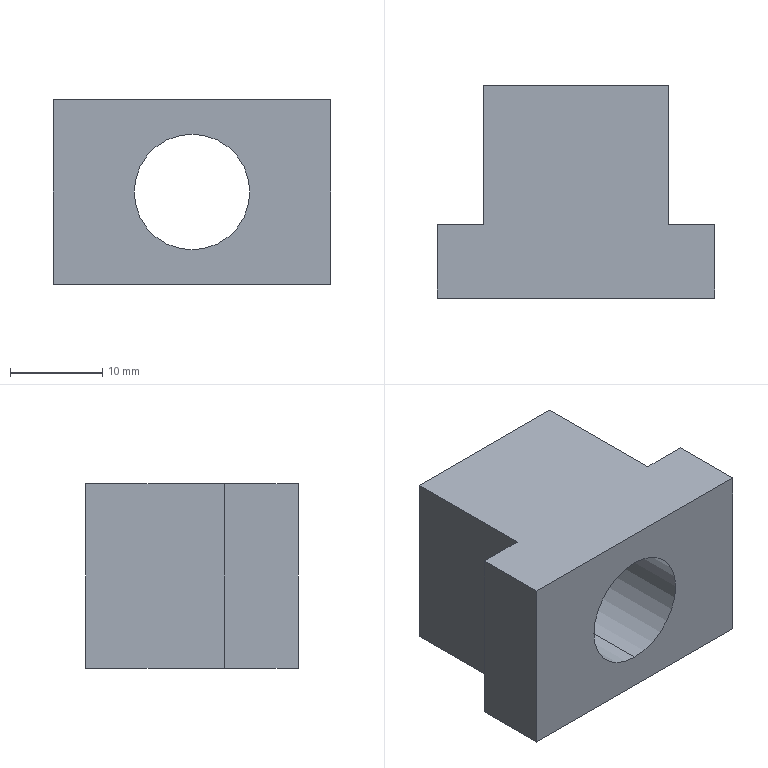Part | STEP file | A14-027 | 1 solid | 12 faces | box 30 x 23 x 20 mm | volume 7977 mm3 | plane 10 | cylinder 2 | commonest cylinder face diameters 12.5 x2
STEP:
#1=CARTESIAN_POINT('',(0.,0.,0.));
#2=DIRECTION('',(0.,0.,1.));
#3=DIRECTION('',(1.,0.,0.));
#4=AXIS2_PLACEMENT_3D('',#1,#2,#3);
#5=CARTESIAN_POINT('',(0.,0.,6.25));
#6=VERTEX_POINT('',#5);
#7=CARTESIAN_POINT('',(0.,23.,6.25));
#8=VERTEX_POINT('',#7);
#9=CARTESIAN_POINT('',(0.,23.,6.25));
#10=DIRECTION('',(0.,1.,0.));
#11=VECTOR('',#10,1.);
#12=LINE('',#9,#11);
#13=CARTESIAN_POINT('',(0.,23.,0.));
#14=DIRECTION('',(0.,1.,0.));
#15=DIRECTION('',(0.,0.,1.));
#16=AXIS2_PLACEMENT_3D('',#13,#14,#15);
#17=CYLINDRICAL_SURFACE('',#16,6.25);
#18=CARTESIAN_POINT('',(6.283,0.));
#19=DIRECTION('',(0.,1.));
#20=VECTOR('',#19,1.);
#21=LINE('',#18,#20);
#22=(GEOMETRIC_REPRESENTATION_CONTEXT(2)PARAMETRIC_REPRESENTATION_CONTEXT()REPRESENTATION_CONTEXT('',''));
#23=DEFINITIONAL_REPRESENTATION('',(#21),#22);
#24=PCURVE('',#17,#23);
#25=CARTESIAN_POINT('',(0.,23.,0.));
#26=DIRECTION('',(0.,1.,0.));
#27=DIRECTION('',(0.,0.,1.));
#28=AXIS2_PLACEMENT_3D('',#25,#26,#27);
#29=CYLINDRICAL_SURFACE('',#28,6.25);
#30=CARTESIAN_POINT('',(0.,0.));
#31=DIRECTION('',(0.,1.));
#32=VECTOR('',#31,1.);
#33=LINE('',#30,#32);
#34=(GEOMETRIC_REPRESENTATION_CONTEXT(2)PARAMETRIC_REPRESENTATION_CONTEXT()REPRESENTATION_CONTEXT('',''));
#35=DEFINITIONAL_REPRESENTATION('',(#33),#34);
#36=PCURVE('',#29,#35);
#37=SURFACE_CURVE('',#12,(#24,#36),.PCURVE_S1.);
#38=EDGE_CURVE('',#6,#8,#37,.T.);
#39=ORIENTED_EDGE('',*,*,#38,.T.);
#40=CARTESIAN_POINT('',(0.,23.,-6.25));
#41=VERTEX_POINT('',#40);
#42=CARTESIAN_POINT('',(0.,23.,0.));
#43=DIRECTION('',(0.,1.,0.));
#44=DIRECTION('',(0.,0.,1.));
#45=AXIS2_PLACEMENT_3D('',#42,#43,#44);
#46=CIRCLE('',#45,6.25);
#47=CARTESIAN_POINT('',(0.,0.));
#48=DIRECTION('',(1.,0.));
#49=VECTOR('',#48,1.);
#50=LINE('',#47,#49);
#51=(GEOMETRIC_REPRESENTATION_CONTEXT(2)PARAMETRIC_REPRESENTATION_CONTEXT()REPRESENTATION_CONTEXT('',''));
#52=DEFINITIONAL_REPRESENTATION('',(#50),#51);
#53=PCURVE('',#17,#52);
#54=CARTESIAN_POINT('',(10.,23.,10.));
#55=DIRECTION('',(0.,-1.,0.));
#56=DIRECTION('',(0.,0.,-1.));
#57=AXIS2_PLACEMENT_3D('',#54,#55,#56);
#58=PLANE('',#57);
#59=CARTESIAN_POINT('',(3.75,-10.));
#60=CARTESIAN_POINT('',(3.75,0.8253));
#61=CARTESIAN_POINT('',(13.125,-4.587));
#62=CARTESIAN_POINT('',(22.5,-10.));
#63=CARTESIAN_POINT('',(13.125,-15.413));
#64=CARTESIAN_POINT('',(3.75,-20.825));
#65=CARTESIAN_POINT('',(3.75,-10.));
#66=(BOUNDED_CURVE()B_SPLINE_CURVE(2,(#59,#60,#61,#62,#63,#64,#65),.UNSPECIFIED.,.T.,.F.)B_SPLINE_CURVE_WITH_KNOTS((1,2,2,2,2,1),(-2.094,0.,2.094,4.189,6.283,8.378),.UNSPECIFIED.)CURVE()GEOMETRIC_REPRESENTATION_ITEM()RATIONAL_B_SPLINE_CURVE((1.,0.5,1.,0.5,1.,0.5,1.))REPRESENTATION_ITEM(''));
#67=(GEOMETRIC_REPRESENTATION_CONTEXT(2)PARAMETRIC_REPRESENTATION_CONTEXT()REPRESENTATION_CONTEXT('',''));
#68=DEFINITIONAL_REPRESENTATION('',(#66),#67);
#69=PCURVE('',#58,#68);
#70=SURFACE_CURVE('',#46,(#53,#69),.PCURVE_S1.);
#71=EDGE_CURVE('',#41,#8,#70,.T.);
#72=ORIENTED_EDGE('',*,*,#71,.F.);
#73=CARTESIAN_POINT('',(0.,0.,-6.25));
#74=VERTEX_POINT('',#73);
#75=CARTESIAN_POINT('',(0.,23.,-6.25));
#76=DIRECTION('',(0.,1.,0.));
#77=VECTOR('',#76,1.);
#78=LINE('',#75,#77);
#79=CARTESIAN_POINT('',(3.142,0.));
#80=DIRECTION('',(0.,1.));
#81=VECTOR('',#80,1.);
#82=LINE('',#79,#81);
#83=(GEOMETRIC_REPRESENTATION_CONTEXT(2)PARAMETRIC_REPRESENTATION_CONTEXT()REPRESENTATION_CONTEXT('',''));
#84=DEFINITIONAL_REPRESENTATION('',(#82),#83);
#85=PCURVE('',#17,#84);
#86=CARTESIAN_POINT('',(3.142,0.));
#87=DIRECTION('',(0.,1.));
#88=VECTOR('',#87,1.);
#89=LINE('',#86,#88);
#90=(GEOMETRIC_REPRESENTATION_CONTEXT(2)PARAMETRIC_REPRESENTATION_CONTEXT()REPRESENTATION_CONTEXT('',''));
#91=DEFINITIONAL_REPRESENTATION('',(#89),#90);
#92=PCURVE('',#29,#91);
#93=SURFACE_CURVE('',#78,(#85,#92),.PCURVE_S1.);
#94=EDGE_CURVE('',#74,#41,#93,.T.);
#95=ORIENTED_EDGE('',*,*,#94,.F.);
#96=CARTESIAN_POINT('',(0.,0.,0.));
#97=DIRECTION('',(0.,1.,0.));
#98=DIRECTION('',(0.,0.,1.));
#99=AXIS2_PLACEMENT_3D('',#96,#97,#98);
#100=CIRCLE('',#99,6.25);
#101=CARTESIAN_POINT('',(0.,-23.));
#102=DIRECTION('',(1.,0.));
#103=VECTOR('',#102,1.);
#104=LINE('',#101,#103);
#105=(GEOMETRIC_REPRESENTATION_CONTEXT(2)PARAMETRIC_REPRESENTATION_CONTEXT()REPRESENTATION_CONTEXT('',''));
#106=DEFINITIONAL_REPRESENTATION('',(#104),#105);
#107=PCURVE('',#17,#106);
#108=CARTESIAN_POINT('',(-15.,0.,10.));
#109=DIRECTION('',(0.,1.,0.));
#110=DIRECTION('',(0.,0.,1.));
#111=AXIS2_PLACEMENT_3D('',#108,#109,#110);
#112=PLANE('',#111);
#113=CARTESIAN_POINT('',(-10.,15.));
#114=DIRECTION('',(1.,0.));
#115=AXIS2_PLACEMENT_2D('',#113,#114);
#116=CIRCLE('',#115,6.25);
#117=(GEOMETRIC_REPRESENTATION_CONTEXT(2)PARAMETRIC_REPRESENTATION_CONTEXT()REPRESENTATION_CONTEXT('',''));
#118=DEFINITIONAL_REPRESENTATION('',(#116),#117);
#119=PCURVE('',#112,#118);
#120=SURFACE_CURVE('',#100,(#107,#119),.PCURVE_S1.);
#121=EDGE_CURVE('',#74,#6,#120,.T.);
#122=ORIENTED_EDGE('',*,*,#121,.T.);
#123=EDGE_LOOP('',(#39,#72,#95,#122));
#124=FACE_BOUND('',#123,.F.);
#125=ADVANCED_FACE('',(#124),#17,.F.);
#126=CARTESIAN_POINT('',(15.,0.,-10.));
#127=VERTEX_POINT('',#126);
#128=CARTESIAN_POINT('',(15.,8.,-10.));
#129=VERTEX_POINT('',#128);
#130=CARTESIAN_POINT('',(15.,0.,-10.));
#131=DIRECTION('',(0.,1.,0.));
#132=VECTOR('',#131,1.);
#133=LINE('',#130,#132);
#134=CARTESIAN_POINT('',(15.,0.,10.));
#135=DIRECTION('',(-1.,0.,0.));
#136=DIRECTION('',(0.,0.,1.));
#137=AXIS2_PLACEMENT_3D('',#134,#135,#136);
#138=PLANE('',#137);
#139=CARTESIAN_POINT('',(-20.,0.));
#140=DIRECTION('',(0.,1.));
#141=VECTOR('',#140,1.);
#142=LINE('',#139,#141);
#143=(GEOMETRIC_REPRESENTATION_CONTEXT(2)PARAMETRIC_REPRESENTATION_CONTEXT()REPRESENTATION_CONTEXT('',''));
#144=DEFINITIONAL_REPRESENTATION('',(#142),#143);
#145=PCURVE('',#138,#144);
#146=CARTESIAN_POINT('',(0.,0.,-10.));
#147=DIRECTION('',(0.,0.,1.));
#148=DIRECTION('',(1.,0.,0.));
#149=AXIS2_PLACEMENT_3D('',#146,#147,#148);
#150=PLANE('',#149);
#151=CARTESIAN_POINT('',(15.,0.));
#152=DIRECTION('',(0.,1.));
#153=VECTOR('',#152,1.);
#154=LINE('',#151,#153);
#155=(GEOMETRIC_REPRESENTATION_CONTEXT(2)PARAMETRIC_REPRESENTATION_CONTEXT()REPRESENTATION_CONTEXT('',''));
#156=DEFINITIONAL_REPRESENTATION('',(#154),#155);
#157=PCURVE('',#150,#156);
#158=SURFACE_CURVE('',#133,(#145,#157),.PCURVE_S1.);
#159=EDGE_CURVE('',#127,#129,#158,.T.);
#160=ORIENTED_EDGE('',*,*,#159,.T.);
#161=CARTESIAN_POINT('',(15.,8.,10.));
#162=VERTEX_POINT('',#161);
#163=CARTESIAN_POINT('',(15.,8.,10.));
#164=DIRECTION('',(0.,0.,-1.));
#165=VECTOR('',#164,1.);
#166=LINE('',#163,#165);
#167=CARTESIAN_POINT('',(0.,8.));
#168=DIRECTION('',(-1.,0.));
#169=VECTOR('',#168,1.);
#170=LINE('',#167,#169);
#171=(GEOMETRIC_REPRESENTATION_CONTEXT(2)PARAMETRIC_REPRESENTATION_CONTEXT()REPRESENTATION_CONTEXT('',''));
#172=DEFINITIONAL_REPRESENTATION('',(#170),#171);
#173=PCURVE('',#138,#172);
#174=CARTESIAN_POINT('',(15.,8.,10.));
#175=DIRECTION('',(0.,-1.,0.));
#176=DIRECTION('',(1.,0.,0.));
#177=AXIS2_PLACEMENT_3D('',#174,#175,#176);
#178=PLANE('',#177);
#179=CARTESIAN_POINT('',(0.,0.));
#180=DIRECTION('',(0.,-1.));
#181=VECTOR('',#180,1.);
#182=LINE('',#179,#181);
#183=(GEOMETRIC_REPRESENTATION_CONTEXT(2)PARAMETRIC_REPRESENTATION_CONTEXT()REPRESENTATION_CONTEXT('',''));
#184=DEFINITIONAL_REPRESENTATION('',(#182),#183);
#185=PCURVE('',#178,#184);
#186=SURFACE_CURVE('',#166,(#173,#185),.PCURVE_S1.);
#187=EDGE_CURVE('',#162,#129,#186,.T.);
#188=ORIENTED_EDGE('',*,*,#187,.F.);
#189=CARTESIAN_POINT('',(15.,0.,10.));
#190=VERTEX_POINT('',#189);
#191=CARTESIAN_POINT('',(15.,0.,10.));
#192=DIRECTION('',(0.,1.,0.));
#193=VECTOR('',#192,1.);
#194=LINE('',#191,#193);
#195=CARTESIAN_POINT('',(0.,0.));
#196=DIRECTION('',(0.,1.));
#197=VECTOR('',#196,1.);
#198=LINE('',#195,#197);
#199=(GEOMETRIC_REPRESENTATION_CONTEXT(2)PARAMETRIC_REPRESENTATION_CONTEXT()REPRESENTATION_CONTEXT('',''));
#200=DEFINITIONAL_REPRESENTATION('',(#198),#199);
#201=PCURVE('',#138,#200);
#202=CARTESIAN_POINT('',(0.,0.,10.));
#203=DIRECTION('',(0.,0.,1.));
#204=DIRECTION('',(1.,0.,0.));
#205=AXIS2_PLACEMENT_3D('',#202,#203,#204);
#206=PLANE('',#205);
#207=CARTESIAN_POINT('',(15.,0.));
#208=DIRECTION('',(0.,1.));
#209=VECTOR('',#208,1.);
#210=LINE('',#207,#209);
#211=(GEOMETRIC_REPRESENTATION_CONTEXT(2)PARAMETRIC_REPRESENTATION_CONTEXT()REPRESENTATION_CONTEXT('',''));
#212=DEFINITIONAL_REPRESENTATION('',(#210),#211);
#213=PCURVE('',#206,#212);
#214=SURFACE_CURVE('',#194,(#201,#213),.PCURVE_S1.);
#215=EDGE_CURVE('',#190,#162,#214,.T.);
#216=ORIENTED_EDGE('',*,*,#215,.F.);
#217=CARTESIAN_POINT('',(15.,0.,10.));
#218=DIRECTION('',(0.,0.,-1.));
#219=VECTOR('',#218,1.);
#220=LINE('',#217,#219);
#221=CARTESIAN_POINT('',(0.,0.));
#222=DIRECTION('',(-1.,0.));
#223=VECTOR('',#222,1.);
#224=LINE('',#221,#223);
#225=(GEOMETRIC_REPRESENTATION_CONTEXT(2)PARAMETRIC_REPRESENTATION_CONTEXT()REPRESENTATION_CONTEXT('',''));
#226=DEFINITIONAL_REPRESENTATION('',(#224),#225);
#227=PCURVE('',#138,#226);
#228=CARTESIAN_POINT('',(0.,30.));
#229=DIRECTION('',(-1.,0.));
#230=VECTOR('',#229,1.);
#231=LINE('',#228,#230);
#232=(GEOMETRIC_REPRESENTATION_CONTEXT(2)PARAMETRIC_REPRESENTATION_CONTEXT()REPRESENTATION_CONTEXT('',''));
#233=DEFINITIONAL_REPRESENTATION('',(#231),#232);
#234=PCURVE('',#112,#233);
#235=SURFACE_CURVE('',#220,(#227,#234),.PCURVE_S1.);
#236=EDGE_CURVE('',#190,#127,#235,.T.);
#237=ORIENTED_EDGE('',*,*,#236,.T.);
#238=EDGE_LOOP('',(#160,#188,#216,#237));
#239=FACE_BOUND('',#238,.T.);
#240=ADVANCED_FACE('',(#239),#138,.F.);
#241=CARTESIAN_POINT('',(10.,8.,-10.));
#242=VERTEX_POINT('',#241);
#243=CARTESIAN_POINT('',(15.,8.,-10.));
#244=DIRECTION('',(-1.,0.,0.));
#245=VECTOR('',#244,1.);
#246=LINE('',#243,#245);
#247=CARTESIAN_POINT('',(0.,-20.));
#248=DIRECTION('',(-1.,0.));
#249=VECTOR('',#248,1.);
#250=LINE('',#247,#249);
#251=(GEOMETRIC_REPRESENTATION_CONTEXT(2)PARAMETRIC_REPRESENTATION_CONTEXT()REPRESENTATION_CONTEXT('',''));
#252=DEFINITIONAL_REPRESENTATION('',(#250),#251);
#253=PCURVE('',#178,#252);
#254=CARTESIAN_POINT('',(15.,8.));
#255=DIRECTION('',(-1.,0.));
#256=VECTOR('',#255,1.);
#257=LINE('',#254,#256);
#258=(GEOMETRIC_REPRESENTATION_CONTEXT(2)PARAMETRIC_REPRESENTATION_CONTEXT()REPRESENTATION_CONTEXT('',''));
#259=DEFINITIONAL_REPRESENTATION('',(#257),#258);
#260=PCURVE('',#150,#259);
#261=SURFACE_CURVE('',#246,(#253,#260),.PCURVE_S1.);
#262=EDGE_CURVE('',#129,#242,#261,.T.);
#263=ORIENTED_EDGE('',*,*,#262,.T.);
#264=CARTESIAN_POINT('',(10.,8.,10.));
#265=VERTEX_POINT('',#264);
#266=CARTESIAN_POINT('',(10.,8.,10.));
#267=DIRECTION('',(0.,0.,-1.));
#268=VECTOR('',#267,1.);
#269=LINE('',#266,#268);
#270=CARTESIAN_POINT('',(-5.,0.));
#271=DIRECTION('',(0.,-1.));
#272=VECTOR('',#271,1.);
#273=LINE('',#270,#272);
#274=(GEOMETRIC_REPRESENTATION_CONTEXT(2)PARAMETRIC_REPRESENTATION_CONTEXT()REPRESENTATION_CONTEXT('',''));
#275=DEFINITIONAL_REPRESENTATION('',(#273),#274);
#276=PCURVE('',#178,#275);
#277=CARTESIAN_POINT('',(10.,8.,10.));
#278=DIRECTION('',(-1.,0.,0.));
#279=DIRECTION('',(0.,0.,1.));
#280=AXIS2_PLACEMENT_3D('',#277,#278,#279);
#281=PLANE('',#280);
#282=CARTESIAN_POINT('',(0.,0.));
#283=DIRECTION('',(-1.,0.));
#284=VECTOR('',#283,1.);
#285=LINE('',#282,#284);
#286=(GEOMETRIC_REPRESENTATION_CONTEXT(2)PARAMETRIC_REPRESENTATION_CONTEXT()REPRESENTATION_CONTEXT('',''));
#287=DEFINITIONAL_REPRESENTATION('',(#285),#286);
#288=PCURVE('',#281,#287);
#289=SURFACE_CURVE('',#269,(#276,#288),.PCURVE_S1.);
#290=EDGE_CURVE('',#265,#242,#289,.T.);
#291=ORIENTED_EDGE('',*,*,#290,.F.);
#292=CARTESIAN_POINT('',(15.,8.,10.));
#293=DIRECTION('',(-1.,0.,0.));
#294=VECTOR('',#293,1.);
#295=LINE('',#292,#294);
#296=CARTESIAN_POINT('',(0.,0.));
#297=DIRECTION('',(-1.,0.));
#298=VECTOR('',#297,1.);
#299=LINE('',#296,#298);
#300=(GEOMETRIC_REPRESENTATION_CONTEXT(2)PARAMETRIC_REPRESENTATION_CONTEXT()REPRESENTATION_CONTEXT('',''));
#301=DEFINITIONAL_REPRESENTATION('',(#299),#300);
#302=PCURVE('',#178,#301);
#303=CARTESIAN_POINT('',(15.,8.));
#304=DIRECTION('',(-1.,0.));
#305=VECTOR('',#304,1.);
#306=LINE('',#303,#305);
#307=(GEOMETRIC_REPRESENTATION_CONTEXT(2)PARAMETRIC_REPRESENTATION_CONTEXT()REPRESENTATION_CONTEXT('',''));
#308=DEFINITIONAL_REPRESENTATION('',(#306),#307);
#309=PCURVE('',#206,#308);
#310=SURFACE_CURVE('',#295,(#302,#309),.PCURVE_S1.);
#311=EDGE_CURVE('',#162,#265,#310,.T.);
#312=ORIENTED_EDGE('',*,*,#311,.F.);
#313=ORIENTED_EDGE('',*,*,#187,.T.);
#314=EDGE_LOOP('',(#263,#291,#312,#313));
#315=FACE_BOUND('',#314,.T.);
#316=ADVANCED_FACE('',(#315),#178,.F.);
#317=CARTESIAN_POINT('',(10.,23.,-10.));
#318=VERTEX_POINT('',#317);
#319=CARTESIAN_POINT('',(10.,8.,-10.));
#320=DIRECTION('',(0.,1.,0.));
#321=VECTOR('',#320,1.);
#322=LINE('',#319,#321);
#323=CARTESIAN_POINT('',(-20.,0.));
#324=DIRECTION('',(0.,1.));
#325=VECTOR('',#324,1.);
#326=LINE('',#323,#325);
#327=(GEOMETRIC_REPRESENTATION_CONTEXT(2)PARAMETRIC_REPRESENTATION_CONTEXT()REPRESENTATION_CONTEXT('',''));
#328=DEFINITIONAL_REPRESENTATION('',(#326),#327);
#329=PCURVE('',#281,#328);
#330=CARTESIAN_POINT('',(10.,8.));
#331=DIRECTION('',(0.,1.));
#332=VECTOR('',#331,1.);
#333=LINE('',#330,#332);
#334=(GEOMETRIC_REPRESENTATION_CONTEXT(2)PARAMETRIC_REPRESENTATION_CONTEXT()REPRESENTATION_CONTEXT('',''));
#335=DEFINITIONAL_REPRESENTATION('',(#333),#334);
#336=PCURVE('',#150,#335);
#337=SURFACE_CURVE('',#322,(#329,#336),.PCURVE_S1.);
#338=EDGE_CURVE('',#242,#318,#337,.T.);
#339=ORIENTED_EDGE('',*,*,#338,.T.);
#340=CARTESIAN_POINT('',(10.,23.,10.));
#341=VERTEX_POINT('',#340);
#342=CARTESIAN_POINT('',(10.,23.,10.));
#343=DIRECTION('',(0.,0.,-1.));
#344=VECTOR('',#343,1.);
#345=LINE('',#342,#344);
#346=CARTESIAN_POINT('',(0.,15.));
#347=DIRECTION('',(-1.,0.));
#348=VECTOR('',#347,1.);
#349=LINE('',#346,#348);
#350=(GEOMETRIC_REPRESENTATION_CONTEXT(2)PARAMETRIC_REPRESENTATION_CONTEXT()REPRESENTATION_CONTEXT('',''));
#351=DEFINITIONAL_REPRESENTATION('',(#349),#350);
#352=PCURVE('',#281,#351);
#353=CARTESIAN_POINT('',(0.,0.));
#354=DIRECTION('',(1.,0.));
#355=VECTOR('',#354,1.);
#356=LINE('',#353,#355);
#357=(GEOMETRIC_REPRESENTATION_CONTEXT(2)PARAMETRIC_REPRESENTATION_CONTEXT()REPRESENTATION_CONTEXT('',''));
#358=DEFINITIONAL_REPRESENTATION('',(#356),#357);
#359=PCURVE('',#58,#358);
#360=SURFACE_CURVE('',#345,(#352,#359),.PCURVE_S1.);
#361=EDGE_CURVE('',#341,#318,#360,.T.);
#362=ORIENTED_EDGE('',*,*,#361,.F.);
#363=CARTESIAN_POINT('',(10.,8.,10.));
#364=DIRECTION('',(0.,1.,0.));
#365=VECTOR('',#364,1.);
#366=LINE('',#363,#365);
#367=CARTESIAN_POINT('',(0.,0.));
#368=DIRECTION('',(0.,1.));
#369=VECTOR('',#368,1.);
#370=LINE('',#367,#369);
#371=(GEOMETRIC_REPRESENTATION_CONTEXT(2)PARAMETRIC_REPRESENTATION_CONTEXT()REPRESENTATION_CONTEXT('',''));
#372=DEFINITIONAL_REPRESENTATION('',(#370),#371);
#373=PCURVE('',#281,#372);
#374=CARTESIAN_POINT('',(10.,8.));
#375=DIRECTION('',(0.,1.));
#376=VECTOR('',#375,1.);
#377=LINE('',#374,#376);
#378=(GEOMETRIC_REPRESENTATION_CONTEXT(2)PARAMETRIC_REPRESENTATION_CONTEXT()REPRESENTATION_CONTEXT('',''));
#379=DEFINITIONAL_REPRESENTATION('',(#377),#378);
#380=PCURVE('',#206,#379);
#381=SURFACE_CURVE('',#366,(#373,#380),.PCURVE_S1.);
#382=EDGE_CURVE('',#265,#341,#381,.T.);
#383=ORIENTED_EDGE('',*,*,#382,.F.);
#384=ORIENTED_EDGE('',*,*,#290,.T.);
#385=EDGE_LOOP('',(#339,#362,#383,#384));
#386=FACE_BOUND('',#385,.T.);
#387=ADVANCED_FACE('',(#386),#281,.F.);
#388=CARTESIAN_POINT('',(0.,23.,0.));
#389=DIRECTION('',(0.,1.,0.));
#390=DIRECTION('',(0.,0.,1.));
#391=AXIS2_PLACEMENT_3D('',#388,#389,#390);
#392=CIRCLE('',#391,6.25);
#393=CARTESIAN_POINT('',(3.75,-10.));
#394=CARTESIAN_POINT('',(3.75,0.8253));
#395=CARTESIAN_POINT('',(13.125,-4.587));
#396=CARTESIAN_POINT('',(22.5,-10.));
#397=CARTESIAN_POINT('',(13.125,-15.413));
#398=CARTESIAN_POINT('',(3.75,-20.825));
#399=CARTESIAN_POINT('',(3.75,-10.));
#400=(BOUNDED_CURVE()B_SPLINE_CURVE(2,(#393,#394,#395,#396,#397,#398,#399),.UNSPECIFIED.,.T.,.F.)B_SPLINE_CURVE_WITH_KNOTS((1,2,2,2,2,1),(-2.094,0.,2.094,4.189,6.283,8.378),.UNSPECIFIED.)CURVE()GEOMETRIC_REPRESENTATION_ITEM()RATIONAL_B_SPLINE_CURVE((1.,0.5,1.,0.5,1.,0.5,1.))REPRESENTATION_ITEM(''));
#401=(GEOMETRIC_REPRESENTATION_CONTEXT(2)PARAMETRIC_REPRESENTATION_CONTEXT()REPRESENTATION_CONTEXT('',''));
#402=DEFINITIONAL_REPRESENTATION('',(#400),#401);
#403=PCURVE('',#58,#402);
#404=CARTESIAN_POINT('',(0.,0.));
#405=DIRECTION('',(1.,0.));
#406=VECTOR('',#405,1.);
#407=LINE('',#404,#406);
#408=(GEOMETRIC_REPRESENTATION_CONTEXT(2)PARAMETRIC_REPRESENTATION_CONTEXT()REPRESENTATION_CONTEXT('',''));
#409=DEFINITIONAL_REPRESENTATION('',(#407),#408);
#410=PCURVE('',#29,#409);
#411=SURFACE_CURVE('',#392,(#403,#410),.PCURVE_S1.);
#412=EDGE_CURVE('',#8,#41,#411,.T.);
#413=ORIENTED_EDGE('',*,*,#412,.F.);
#414=ORIENTED_EDGE('',*,*,#71,.F.);
#415=EDGE_LOOP('',(#413,#414));
#416=FACE_BOUND('',#415,.T.);
#417=CARTESIAN_POINT('',(-10.,23.,-10.));
#418=VERTEX_POINT('',#417);
#419=CARTESIAN_POINT('',(10.,23.,-10.));
#420=DIRECTION('',(-1.,0.,0.));
#421=VECTOR('',#420,1.);
#422=LINE('',#419,#421);
#423=CARTESIAN_POINT('',(20.,0.));
#424=DIRECTION('',(0.,-1.));
#425=VECTOR('',#424,1.);
#426=LINE('',#423,#425);
#427=(GEOMETRIC_REPRESENTATION_CONTEXT(2)PARAMETRIC_REPRESENTATION_CONTEXT()REPRESENTATION_CONTEXT('',''));
#428=DEFINITIONAL_REPRESENTATION('',(#426),#427);
#429=PCURVE('',#58,#428);
#430=CARTESIAN_POINT('',(10.,23.));
#431=DIRECTION('',(-1.,0.));
#432=VECTOR('',#431,1.);
#433=LINE('',#430,#432);
#434=(GEOMETRIC_REPRESENTATION_CONTEXT(2)PARAMETRIC_REPRESENTATION_CONTEXT()REPRESENTATION_CONTEXT('',''));
#435=DEFINITIONAL_REPRESENTATION('',(#433),#434);
#436=PCURVE('',#150,#435);
#437=SURFACE_CURVE('',#422,(#429,#436),.PCURVE_S1.);
#438=EDGE_CURVE('',#318,#418,#437,.T.);
#439=ORIENTED_EDGE('',*,*,#438,.T.);
#440=CARTESIAN_POINT('',(-10.,23.,10.));
#441=VERTEX_POINT('',#440);
#442=CARTESIAN_POINT('',(-10.,23.,10.));
#443=DIRECTION('',(0.,0.,-1.));
#444=VECTOR('',#443,1.);
#445=LINE('',#442,#444);
#446=CARTESIAN_POINT('',(0.,-20.));
#447=DIRECTION('',(1.,0.));
#448=VECTOR('',#447,1.);
#449=LINE('',#446,#448);
#450=(GEOMETRIC_REPRESENTATION_CONTEXT(2)PARAMETRIC_REPRESENTATION_CONTEXT()REPRESENTATION_CONTEXT('',''));
#451=DEFINITIONAL_REPRESENTATION('',(#449),#450);
#452=PCURVE('',#58,#451);
#453=CARTESIAN_POINT('',(-10.,23.,10.));
#454=DIRECTION('',(1.,0.,0.));
#455=DIRECTION('',(0.,1.,0.));
#456=AXIS2_PLACEMENT_3D('',#453,#454,#455);
#457=PLANE('',#456);
#458=CARTESIAN_POINT('',(0.,0.));
#459=DIRECTION('',(0.,-1.));
#460=VECTOR('',#459,1.);
#461=LINE('',#458,#460);
#462=(GEOMETRIC_REPRESENTATION_CONTEXT(2)PARAMETRIC_REPRESENTATION_CONTEXT()REPRESENTATION_CONTEXT('',''));
#463=DEFINITIONAL_REPRESENTATION('',(#461),#462);
#464=PCURVE('',#457,#463);
#465=SURFACE_CURVE('',#445,(#452,#464),.PCURVE_S1.);
#466=EDGE_CURVE('',#441,#418,#465,.T.);
#467=ORIENTED_EDGE('',*,*,#466,.F.);
#468=CARTESIAN_POINT('',(10.,23.,10.));
#469=DIRECTION('',(-1.,0.,0.));
#470=VECTOR('',#469,1.);
#471=LINE('',#468,#470);
#472=CARTESIAN_POINT('',(0.,0.));
#473=DIRECTION('',(0.,-1.));
#474=VECTOR('',#473,1.);
#475=LINE('',#472,#474);
#476=(GEOMETRIC_REPRESENTATION_CONTEXT(2)PARAMETRIC_REPRESENTATION_CONTEXT()REPRESENTATION_CONTEXT('',''));
#477=DEFINITIONAL_REPRESENTATION('',(#475),#476);
#478=PCURVE('',#58,#477);
#479=CARTESIAN_POINT('',(10.,23.));
#480=DIRECTION('',(-1.,0.));
#481=VECTOR('',#480,1.);
#482=LINE('',#479,#481);
#483=(GEOMETRIC_REPRESENTATION_CONTEXT(2)PARAMETRIC_REPRESENTATION_CONTEXT()REPRESENTATION_CONTEXT('',''));
#484=DEFINITIONAL_REPRESENTATION('',(#482),#483);
#485=PCURVE('',#206,#484);
#486=SURFACE_CURVE('',#471,(#478,#485),.PCURVE_S1.);
#487=EDGE_CURVE('',#341,#441,#486,.T.);
#488=ORIENTED_EDGE('',*,*,#487,.F.);
#489=ORIENTED_EDGE('',*,*,#361,.T.);
#490=EDGE_LOOP('',(#439,#467,#488,#489));
#491=FACE_BOUND('',#490,.T.);
#492=ADVANCED_FACE('',(#416,#491),#58,.F.);
#493=CARTESIAN_POINT('',(-10.,8.,-10.));
#494=VERTEX_POINT('',#493);
#495=CARTESIAN_POINT('',(-10.,23.,-10.));
#496=DIRECTION('',(0.,-1.,0.));
#497=VECTOR('',#496,1.);
#498=LINE('',#495,#497);
#499=CARTESIAN_POINT('',(0.,-20.));
#500=DIRECTION('',(-1.,0.));
#501=VECTOR('',#500,1.);
#502=LINE('',#499,#501);
#503=(GEOMETRIC_REPRESENTATION_CONTEXT(2)PARAMETRIC_REPRESENTATION_CONTEXT()REPRESENTATION_CONTEXT('',''));
#504=DEFINITIONAL_REPRESENTATION('',(#502),#503);
#505=PCURVE('',#457,#504);
#506=CARTESIAN_POINT('',(-10.,23.));
#507=DIRECTION('',(0.,-1.));
#508=VECTOR('',#507,1.);
#509=LINE('',#506,#508);
#510=(GEOMETRIC_REPRESENTATION_CONTEXT(2)PARAMETRIC_REPRESENTATION_CONTEXT()REPRESENTATION_CONTEXT('',''));
#511=DEFINITIONAL_REPRESENTATION('',(#509),#510);
#512=PCURVE('',#150,#511);
#513=SURFACE_CURVE('',#498,(#505,#512),.PCURVE_S1.);
#514=EDGE_CURVE('',#418,#494,#513,.T.);
#515=ORIENTED_EDGE('',*,*,#514,.T.);
#516=CARTESIAN_POINT('',(-10.,8.,10.));
#517=VERTEX_POINT('',#516);
#518=CARTESIAN_POINT('',(-10.,8.,10.));
#519=DIRECTION('',(0.,0.,-1.));
#520=VECTOR('',#519,1.);
#521=LINE('',#518,#520);
#522=CARTESIAN_POINT('',(-15.,0.));
#523=DIRECTION('',(0.,-1.));
#524=VECTOR('',#523,1.);
#525=LINE('',#522,#524);
#526=(GEOMETRIC_REPRESENTATION_CONTEXT(2)PARAMETRIC_REPRESENTATION_CONTEXT()REPRESENTATION_CONTEXT('',''));
#527=DEFINITIONAL_REPRESENTATION('',(#525),#526);
#528=PCURVE('',#457,#527);
#529=CARTESIAN_POINT('',(-10.,8.,10.));
#530=DIRECTION('',(0.,-1.,0.));
#531=DIRECTION('',(1.,0.,0.));
#532=AXIS2_PLACEMENT_3D('',#529,#530,#531);
#533=PLANE('',#532);
#534=CARTESIAN_POINT('',(0.,0.));
#535=DIRECTION('',(0.,-1.));
#536=VECTOR('',#535,1.);
#537=LINE('',#534,#536);
#538=(GEOMETRIC_REPRESENTATION_CONTEXT(2)PARAMETRIC_REPRESENTATION_CONTEXT()REPRESENTATION_CONTEXT('',''));
#539=DEFINITIONAL_REPRESENTATION('',(#537),#538);
#540=PCURVE('',#533,#539);
#541=SURFACE_CURVE('',#521,(#528,#540),.PCURVE_S1.);
#542=EDGE_CURVE('',#517,#494,#541,.T.);
#543=ORIENTED_EDGE('',*,*,#542,.F.);
#544=CARTESIAN_POINT('',(-10.,23.,10.));
#545=DIRECTION('',(0.,-1.,0.));
#546=VECTOR('',#545,1.);
#547=LINE('',#544,#546);
#548=CARTESIAN_POINT('',(0.,0.));
#549=DIRECTION('',(-1.,0.));
#550=VECTOR('',#549,1.);
#551=LINE('',#548,#550);
#552=(GEOMETRIC_REPRESENTATION_CONTEXT(2)PARAMETRIC_REPRESENTATION_CONTEXT()REPRESENTATION_CONTEXT('',''));
#553=DEFINITIONAL_REPRESENTATION('',(#551),#552);
#554=PCURVE('',#457,#553);
#555=CARTESIAN_POINT('',(-10.,23.));
#556=DIRECTION('',(0.,-1.));
#557=VECTOR('',#556,1.);
#558=LINE('',#555,#557);
#559=(GEOMETRIC_REPRESENTATION_CONTEXT(2)PARAMETRIC_REPRESENTATION_CONTEXT()REPRESENTATION_CONTEXT('',''));
#560=DEFINITIONAL_REPRESENTATION('',(#558),#559);
#561=PCURVE('',#206,#560);
#562=SURFACE_CURVE('',#547,(#554,#561),.PCURVE_S1.);
#563=EDGE_CURVE('',#441,#517,#562,.T.);
#564=ORIENTED_EDGE('',*,*,#563,.F.);
#565=ORIENTED_EDGE('',*,*,#466,.T.);
#566=EDGE_LOOP('',(#515,#543,#564,#565));
#567=FACE_BOUND('',#566,.T.);
#568=ADVANCED_FACE('',(#567),#457,.F.);
#569=CARTESIAN_POINT('',(-15.,8.,-10.));
#570=VERTEX_POINT('',#569);
#571=CARTESIAN_POINT('',(-10.,8.,-10.));
#572=DIRECTION('',(-1.,0.,0.));
#573=VECTOR('',#572,1.);
#574=LINE('',#571,#573);
#575=CARTESIAN_POINT('',(0.,-20.));
#576=DIRECTION('',(-1.,0.));
#577=VECTOR('',#576,1.);
#578=LINE('',#575,#577);
#579=(GEOMETRIC_REPRESENTATION_CONTEXT(2)PARAMETRIC_REPRESENTATION_CONTEXT()REPRESENTATION_CONTEXT('',''));
#580=DEFINITIONAL_REPRESENTATION('',(#578),#579);
#581=PCURVE('',#533,#580);
#582=CARTESIAN_POINT('',(-10.,8.));
#583=DIRECTION('',(-1.,0.));
#584=VECTOR('',#583,1.);
#585=LINE('',#582,#584);
#586=(GEOMETRIC_REPRESENTATION_CONTEXT(2)PARAMETRIC_REPRESENTATION_CONTEXT()REPRESENTATION_CONTEXT('',''));
#587=DEFINITIONAL_REPRESENTATION('',(#585),#586);
#588=PCURVE('',#150,#587);
#589=SURFACE_CURVE('',#574,(#581,#588),.PCURVE_S1.);
#590=EDGE_CURVE('',#494,#570,#589,.T.);
#591=ORIENTED_EDGE('',*,*,#590,.T.);
#592=CARTESIAN_POINT('',(-15.,8.,10.));
#593=VERTEX_POINT('',#592);
#594=CARTESIAN_POINT('',(-15.,8.,10.));
#595=DIRECTION('',(0.,0.,-1.));
#596=VECTOR('',#595,1.);
#597=LINE('',#594,#596);
#598=CARTESIAN_POINT('',(-5.,0.));
#599=DIRECTION('',(0.,-1.));
#600=VECTOR('',#599,1.);
#601=LINE('',#598,#600);
#602=(GEOMETRIC_REPRESENTATION_CONTEXT(2)PARAMETRIC_REPRESENTATION_CONTEXT()REPRESENTATION_CONTEXT('',''));
#603=DEFINITIONAL_REPRESENTATION('',(#601),#602);
#604=PCURVE('',#533,#603);
#605=CARTESIAN_POINT('',(-15.,8.,10.));
#606=DIRECTION('',(1.,0.,0.));
#607=DIRECTION('',(0.,1.,0.));
#608=AXIS2_PLACEMENT_3D('',#605,#606,#607);
#609=PLANE('',#608);
#610=CARTESIAN_POINT('',(0.,0.));
#611=DIRECTION('',(0.,-1.));
#612=VECTOR('',#611,1.);
#613=LINE('',#610,#612);
#614=(GEOMETRIC_REPRESENTATION_CONTEXT(2)PARAMETRIC_REPRESENTATION_CONTEXT()REPRESENTATION_CONTEXT('',''));
#615=DEFINITIONAL_REPRESENTATION('',(#613),#614);
#616=PCURVE('',#609,#615);
#617=SURFACE_CURVE('',#597,(#604,#616),.PCURVE_S1.);
#618=EDGE_CURVE('',#593,#570,#617,.T.);
#619=ORIENTED_EDGE('',*,*,#618,.F.);
#620=CARTESIAN_POINT('',(-10.,8.,10.));
#621=DIRECTION('',(-1.,0.,0.));
#622=VECTOR('',#621,1.);
#623=LINE('',#620,#622);
#624=CARTESIAN_POINT('',(0.,0.));
#625=DIRECTION('',(-1.,0.));
#626=VECTOR('',#625,1.);
#627=LINE('',#624,#626);
#628=(GEOMETRIC_REPRESENTATION_CONTEXT(2)PARAMETRIC_REPRESENTATION_CONTEXT()REPRESENTATION_CONTEXT('',''));
#629=DEFINITIONAL_REPRESENTATION('',(#627),#628);
#630=PCURVE('',#533,#629);
#631=CARTESIAN_POINT('',(-10.,8.));
#632=DIRECTION('',(-1.,0.));
#633=VECTOR('',#632,1.);
#634=LINE('',#631,#633);
#635=(GEOMETRIC_REPRESENTATION_CONTEXT(2)PARAMETRIC_REPRESENTATION_CONTEXT()REPRESENTATION_CONTEXT('',''));
#636=DEFINITIONAL_REPRESENTATION('',(#634),#635);
#637=PCURVE('',#206,#636);
#638=SURFACE_CURVE('',#623,(#630,#637),.PCURVE_S1.);
#639=EDGE_CURVE('',#517,#593,#638,.T.);
#640=ORIENTED_EDGE('',*,*,#639,.F.);
#641=ORIENTED_EDGE('',*,*,#542,.T.);
#642=EDGE_LOOP('',(#591,#619,#640,#641));
#643=FACE_BOUND('',#642,.T.);
#644=ADVANCED_FACE('',(#643),#533,.F.);
#645=CARTESIAN_POINT('',(-15.,0.,-10.));
#646=VERTEX_POINT('',#645);
#647=CARTESIAN_POINT('',(-15.,8.,-10.));
#648=DIRECTION('',(0.,-1.,0.));
#649=VECTOR('',#648,1.);
#650=LINE('',#647,#649);
#651=CARTESIAN_POINT('',(0.,-20.));
#652=DIRECTION('',(-1.,0.));
#653=VECTOR('',#652,1.);
#654=LINE('',#651,#653);
#655=(GEOMETRIC_REPRESENTATION_CONTEXT(2)PARAMETRIC_REPRESENTATION_CONTEXT()REPRESENTATION_CONTEXT('',''));
#656=DEFINITIONAL_REPRESENTATION('',(#654),#655);
#657=PCURVE('',#609,#656);
#658=CARTESIAN_POINT('',(-15.,8.));
#659=DIRECTION('',(0.,-1.));
#660=VECTOR('',#659,1.);
#661=LINE('',#658,#660);
#662=(GEOMETRIC_REPRESENTATION_CONTEXT(2)PARAMETRIC_REPRESENTATION_CONTEXT()REPRESENTATION_CONTEXT('',''));
#663=DEFINITIONAL_REPRESENTATION('',(#661),#662);
#664=PCURVE('',#150,#663);
#665=SURFACE_CURVE('',#650,(#657,#664),.PCURVE_S1.);
#666=EDGE_CURVE('',#570,#646,#665,.T.);
#667=ORIENTED_EDGE('',*,*,#666,.T.);
#668=CARTESIAN_POINT('',(-15.,0.,10.));
#669=VERTEX_POINT('',#668);
#670=CARTESIAN_POINT('',(-15.,0.,10.));
#671=DIRECTION('',(0.,0.,-1.));
#672=VECTOR('',#671,1.);
#673=LINE('',#670,#672);
#674=CARTESIAN_POINT('',(-8.,0.));
#675=DIRECTION('',(0.,-1.));
#676=VECTOR('',#675,1.);
#677=LINE('',#674,#676);
#678=(GEOMETRIC_REPRESENTATION_CONTEXT(2)PARAMETRIC_REPRESENTATION_CONTEXT()REPRESENTATION_CONTEXT('',''));
#679=DEFINITIONAL_REPRESENTATION('',(#677),#678);
#680=PCURVE('',#609,#679);
#681=CARTESIAN_POINT('',(0.,0.));
#682=DIRECTION('',(-1.,0.));
#683=VECTOR('',#682,1.);
#684=LINE('',#681,#683);
#685=(GEOMETRIC_REPRESENTATION_CONTEXT(2)PARAMETRIC_REPRESENTATION_CONTEXT()REPRESENTATION_CONTEXT('',''));
#686=DEFINITIONAL_REPRESENTATION('',(#684),#685);
#687=PCURVE('',#112,#686);
#688=SURFACE_CURVE('',#673,(#680,#687),.PCURVE_S1.);
#689=EDGE_CURVE('',#669,#646,#688,.T.);
#690=ORIENTED_EDGE('',*,*,#689,.F.);
#691=CARTESIAN_POINT('',(-15.,8.,10.));
#692=DIRECTION('',(0.,-1.,0.));
#693=VECTOR('',#692,1.);
#694=LINE('',#691,#693);
#695=CARTESIAN_POINT('',(0.,0.));
#696=DIRECTION('',(-1.,0.));
#697=VECTOR('',#696,1.);
#698=LINE('',#695,#697);
#699=(GEOMETRIC_REPRESENTATION_CONTEXT(2)PARAMETRIC_REPRESENTATION_CONTEXT()REPRESENTATION_CONTEXT('',''));
#700=DEFINITIONAL_REPRESENTATION('',(#698),#699);
#701=PCURVE('',#609,#700);
#702=CARTESIAN_POINT('',(-15.,8.));
#703=DIRECTION('',(0.,-1.));
#704=VECTOR('',#703,1.);
#705=LINE('',#702,#704);
#706=(GEOMETRIC_REPRESENTATION_CONTEXT(2)PARAMETRIC_REPRESENTATION_CONTEXT()REPRESENTATION_CONTEXT('',''));
#707=DEFINITIONAL_REPRESENTATION('',(#705),#706);
#708=PCURVE('',#206,#707);
#709=SURFACE_CURVE('',#694,(#701,#708),.PCURVE_S1.);
#710=EDGE_CURVE('',#593,#669,#709,.T.);
#711=ORIENTED_EDGE('',*,*,#710,.F.);
#712=ORIENTED_EDGE('',*,*,#618,.T.);
#713=EDGE_LOOP('',(#667,#690,#711,#712));
#714=FACE_BOUND('',#713,.T.);
#715=ADVANCED_FACE('',(#714),#609,.F.);
#716=CARTESIAN_POINT('',(0.,0.,0.));
#717=DIRECTION('',(0.,1.,0.));
#718=DIRECTION('',(0.,0.,1.));
#719=AXIS2_PLACEMENT_3D('',#716,#717,#718);
#720=CIRCLE('',#719,6.25);
#721=CARTESIAN_POINT('',(-10.,15.));
#722=DIRECTION('',(1.,0.));
#723=AXIS2_PLACEMENT_2D('',#721,#722);
#724=CIRCLE('',#723,6.25);
#725=(GEOMETRIC_REPRESENTATION_CONTEXT(2)PARAMETRIC_REPRESENTATION_CONTEXT()REPRESENTATION_CONTEXT('',''));
#726=DEFINITIONAL_REPRESENTATION('',(#724),#725);
#727=PCURVE('',#112,#726);
#728=CARTESIAN_POINT('',(0.,-23.));
#729=DIRECTION('',(1.,0.));
#730=VECTOR('',#729,1.);
#731=LINE('',#728,#730);
#732=(GEOMETRIC_REPRESENTATION_CONTEXT(2)PARAMETRIC_REPRESENTATION_CONTEXT()REPRESENTATION_CONTEXT('',''));
#733=DEFINITIONAL_REPRESENTATION('',(#731),#732);
#734=PCURVE('',#29,#733);
#735=SURFACE_CURVE('',#720,(#727,#734),.PCURVE_S1.);
#736=EDGE_CURVE('',#6,#74,#735,.T.);
#737=ORIENTED_EDGE('',*,*,#736,.T.);
#738=ORIENTED_EDGE('',*,*,#121,.T.);
#739=EDGE_LOOP('',(#737,#738));
#740=FACE_BOUND('',#739,.T.);
#741=CARTESIAN_POINT('',(-15.,0.,-10.));
#742=DIRECTION('',(1.,0.,0.));
#743=VECTOR('',#742,1.);
#744=LINE('',#741,#743);
#745=CARTESIAN_POINT('',(-20.,0.));
#746=DIRECTION('',(0.,1.));
#747=VECTOR('',#746,1.);
#748=LINE('',#745,#747);
#749=(GEOMETRIC_REPRESENTATION_CONTEXT(2)PARAMETRIC_REPRESENTATION_CONTEXT()REPRESENTATION_CONTEXT('',''));
#750=DEFINITIONAL_REPRESENTATION('',(#748),#749);
#751=PCURVE('',#112,#750);
#752=CARTESIAN_POINT('',(-15.,0.));
#753=DIRECTION('',(1.,0.));
#754=VECTOR('',#753,1.);
#755=LINE('',#752,#754);
#756=(GEOMETRIC_REPRESENTATION_CONTEXT(2)PARAMETRIC_REPRESENTATION_CONTEXT()REPRESENTATION_CONTEXT('',''));
#757=DEFINITIONAL_REPRESENTATION('',(#755),#756);
#758=PCURVE('',#150,#757);
#759=SURFACE_CURVE('',#744,(#751,#758),.PCURVE_S1.);
#760=EDGE_CURVE('',#646,#127,#759,.T.);
#761=ORIENTED_EDGE('',*,*,#760,.T.);
#762=ORIENTED_EDGE('',*,*,#236,.F.);
#763=CARTESIAN_POINT('',(-15.,0.,10.));
#764=DIRECTION('',(1.,0.,0.));
#765=VECTOR('',#764,1.);
#766=LINE('',#763,#765);
#767=CARTESIAN_POINT('',(0.,0.));
#768=DIRECTION('',(0.,1.));
#769=VECTOR('',#768,1.);
#770=LINE('',#767,#769);
#771=(GEOMETRIC_REPRESENTATION_CONTEXT(2)PARAMETRIC_REPRESENTATION_CONTEXT()REPRESENTATION_CONTEXT('',''));
#772=DEFINITIONAL_REPRESENTATION('',(#770),#771);
#773=PCURVE('',#112,#772);
#774=CARTESIAN_POINT('',(-15.,0.));
#775=DIRECTION('',(1.,0.));
#776=VECTOR('',#775,1.);
#777=LINE('',#774,#776);
#778=(GEOMETRIC_REPRESENTATION_CONTEXT(2)PARAMETRIC_REPRESENTATION_CONTEXT()REPRESENTATION_CONTEXT('',''));
#779=DEFINITIONAL_REPRESENTATION('',(#777),#778);
#780=PCURVE('',#206,#779);
#781=SURFACE_CURVE('',#766,(#773,#780),.PCURVE_S1.);
#782=EDGE_CURVE('',#669,#190,#781,.T.);
#783=ORIENTED_EDGE('',*,*,#782,.F.);
#784=ORIENTED_EDGE('',*,*,#689,.T.);
#785=EDGE_LOOP('',(#761,#762,#783,#784));
#786=FACE_BOUND('',#785,.T.);
#787=ADVANCED_FACE('',(#740,#786),#112,.F.);
#788=ORIENTED_EDGE('',*,*,#215,.T.);
#789=ORIENTED_EDGE('',*,*,#311,.T.);
#790=ORIENTED_EDGE('',*,*,#382,.T.);
#791=ORIENTED_EDGE('',*,*,#487,.T.);
#792=ORIENTED_EDGE('',*,*,#563,.T.);
#793=ORIENTED_EDGE('',*,*,#639,.T.);
#794=ORIENTED_EDGE('',*,*,#710,.T.);
#795=ORIENTED_EDGE('',*,*,#782,.T.);
#796=EDGE_LOOP('',(#788,#789,#790,#791,#792,#793,#794,#795));
#797=FACE_BOUND('',#796,.T.);
#798=ADVANCED_FACE('',(#797),#206,.T.);
#799=ORIENTED_EDGE('',*,*,#159,.F.);
#800=ORIENTED_EDGE('',*,*,#760,.F.);
#801=ORIENTED_EDGE('',*,*,#666,.F.);
#802=ORIENTED_EDGE('',*,*,#590,.F.);
#803=ORIENTED_EDGE('',*,*,#514,.F.);
#804=ORIENTED_EDGE('',*,*,#438,.F.);
#805=ORIENTED_EDGE('',*,*,#338,.F.);
#806=ORIENTED_EDGE('',*,*,#262,.F.);
#807=EDGE_LOOP('',(#799,#800,#801,#802,#803,#804,#805,#806));
#808=FACE_BOUND('',#807,.T.);
#809=ADVANCED_FACE('',(#808),#150,.F.);
#810=ORIENTED_EDGE('',*,*,#412,.F.);
#811=ORIENTED_EDGE('',*,*,#38,.F.);
#812=ORIENTED_EDGE('',*,*,#736,.T.);
#813=ORIENTED_EDGE('',*,*,#94,.T.);
#814=EDGE_LOOP('',(#810,#811,#812,#813));
#815=FACE_BOUND('',#814,.F.);
#816=ADVANCED_FACE('',(#815),#29,.F.);
#817=CLOSED_SHELL('',(#125,#240,#316,#387,#492,#568,#644,#715,#787,#798,#809,#816));
#818=MANIFOLD_SOLID_BREP('',#817);
#819=(LENGTH_UNIT()NAMED_UNIT(*)SI_UNIT(.MILLI.,.METRE.));
#820=UNCERTAINTY_MEASURE_WITH_UNIT(LENGTH_MEASURE(0.0000001),#819,'','');
#821=(NAMED_UNIT(*)PLANE_ANGLE_UNIT()SI_UNIT($,.RADIAN.));
#822=(NAMED_UNIT(*)SI_UNIT($,.STERADIAN.)SOLID_ANGLE_UNIT());
#823=(GEOMETRIC_REPRESENTATION_CONTEXT(3)GLOBAL_UNCERTAINTY_ASSIGNED_CONTEXT((#820))GLOBAL_UNIT_ASSIGNED_CONTEXT((#819,#821,#822))REPRESENTATION_CONTEXT('',''));
#824=ADVANCED_BREP_SHAPE_REPRESENTATION('',(#4,#818),#823);